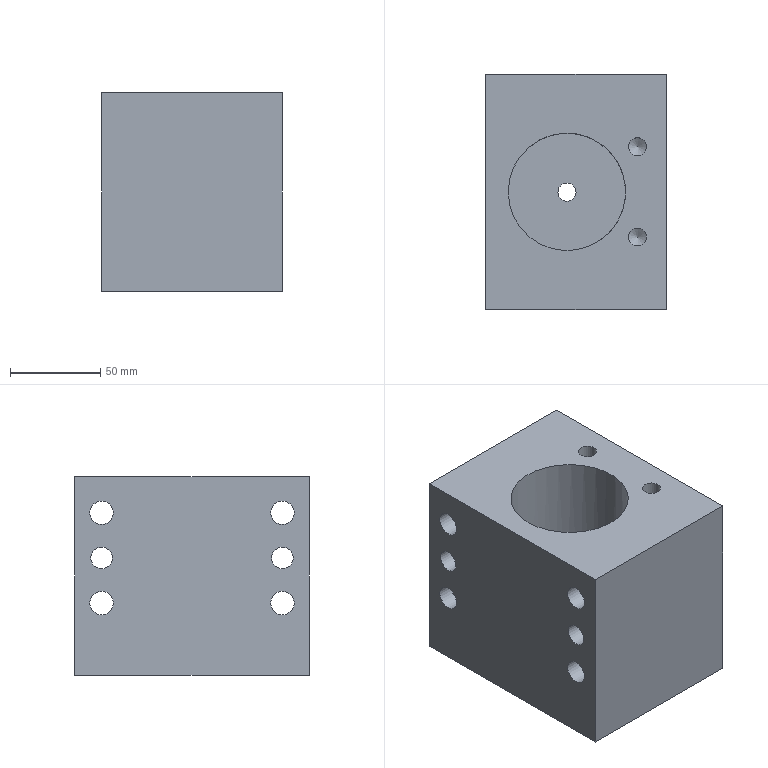Part | NX | features solid 2 | 1 solid | 31 faces | box 100 x 130 x 110 mm | volume 972878 mm3 | cylinder 16 | plane 13 | cone 2 | commonest cylinder face diameters 13 x4 20 x4 10 x3 12 x2 14 x2 65 x1
STEP:
#1=CARTESIAN_POINT('',(670.,65.,-145.));
#2=VERTEX_POINT('',#1);
#3=CARTESIAN_POINT('',(670.,65.,-152.));
#4=DIRECTION('',(-1.,0.,0.));
#5=DIRECTION('',(0.,0.,1.));
#6=AXIS2_PLACEMENT_3D('',#3,#4,#5);
#7=CIRCLE('',#6,7.);
#8=EDGE_CURVE('',#2,#2,#7,.F.);
#9=ORIENTED_EDGE('',*,*,#8,.F.);
#10=EDGE_LOOP('',(#9));
#11=FACE_BOUND('',#10,.T.);
#12=CARTESIAN_POINT('',(670.,165.,-117.));
#13=VERTEX_POINT('',#12);
#14=CARTESIAN_POINT('',(670.,165.,-127.));
#15=DIRECTION('',(-1.,0.,0.));
#16=DIRECTION('',(0.,0.,1.));
#17=AXIS2_PLACEMENT_3D('',#14,#15,#16);
#18=CIRCLE('',#17,10.);
#19=EDGE_CURVE('',#13,#13,#18,.T.);
#20=ORIENTED_EDGE('',*,*,#19,.T.);
#21=EDGE_LOOP('',(#20));
#22=FACE_BOUND('',#21,.T.);
#23=CARTESIAN_POINT('',(670.,165.,-167.));
#24=VERTEX_POINT('',#23);
#25=CARTESIAN_POINT('',(670.,165.,-177.));
#26=DIRECTION('',(-1.,0.,0.));
#27=DIRECTION('',(0.,0.,1.));
#28=AXIS2_PLACEMENT_3D('',#25,#26,#27);
#29=CIRCLE('',#28,10.);
#30=EDGE_CURVE('',#24,#24,#29,.T.);
#31=ORIENTED_EDGE('',*,*,#30,.T.);
#32=EDGE_LOOP('',(#31));
#33=FACE_BOUND('',#32,.T.);
#34=CARTESIAN_POINT('',(670.,65.,-167.));
#35=VERTEX_POINT('',#34);
#36=CARTESIAN_POINT('',(670.,65.,-177.));
#37=DIRECTION('',(-1.,0.,0.));
#38=DIRECTION('',(0.,0.,1.));
#39=AXIS2_PLACEMENT_3D('',#36,#37,#38);
#40=CIRCLE('',#39,10.);
#41=EDGE_CURVE('',#35,#35,#40,.T.);
#42=ORIENTED_EDGE('',*,*,#41,.T.);
#43=EDGE_LOOP('',(#42));
#44=FACE_BOUND('',#43,.T.);
#45=CARTESIAN_POINT('',(670.,65.,-117.));
#46=VERTEX_POINT('',#45);
#47=CARTESIAN_POINT('',(670.,65.,-127.));
#48=DIRECTION('',(-1.,0.,0.));
#49=DIRECTION('',(0.,0.,1.));
#50=AXIS2_PLACEMENT_3D('',#47,#48,#49);
#51=CIRCLE('',#50,10.);
#52=EDGE_CURVE('',#46,#46,#51,.T.);
#53=ORIENTED_EDGE('',*,*,#52,.T.);
#54=EDGE_LOOP('',(#53));
#55=FACE_BOUND('',#54,.T.);
#56=CARTESIAN_POINT('',(670.,180.,-107.));
#57=VERTEX_POINT('',#56);
#58=CARTESIAN_POINT('',(670.,50.,-107.));
#59=VERTEX_POINT('',#58);
#60=CARTESIAN_POINT('',(670.,180.,-107.));
#61=DIRECTION('',(0.,-1.,0.));
#62=VECTOR('',#61,1000.);
#63=LINE('',#60,#62);
#64=EDGE_CURVE('',#57,#59,#63,.T.);
#65=ORIENTED_EDGE('',*,*,#64,.T.);
#66=CARTESIAN_POINT('',(670.,50.,-217.));
#67=VERTEX_POINT('',#66);
#68=CARTESIAN_POINT('',(670.,50.,-210.));
#69=DIRECTION('',(0.,0.,1.));
#70=VECTOR('',#69,1000.);
#71=LINE('',#68,#70);
#72=EDGE_CURVE('',#67,#59,#71,.T.);
#73=ORIENTED_EDGE('',*,*,#72,.F.);
#74=CARTESIAN_POINT('',(670.,180.,-217.));
#75=VERTEX_POINT('',#74);
#76=CARTESIAN_POINT('',(670.,180.,-217.));
#77=DIRECTION('',(0.,1.,0.));
#78=VECTOR('',#77,1000.);
#79=LINE('',#76,#78);
#80=EDGE_CURVE('',#75,#67,#79,.F.);
#81=ORIENTED_EDGE('',*,*,#80,.F.);
#82=CARTESIAN_POINT('',(670.,180.,-210.));
#83=DIRECTION('',(0.,0.,1.));
#84=VECTOR('',#83,1000.);
#85=LINE('',#82,#84);
#86=EDGE_CURVE('',#75,#57,#85,.T.);
#87=ORIENTED_EDGE('',*,*,#86,.T.);
#88=EDGE_LOOP('',(#65,#73,#81,#87));
#89=FACE_BOUND('',#88,.T.);
#90=CARTESIAN_POINT('',(670.,165.,-145.));
#91=VERTEX_POINT('',#90);
#92=CARTESIAN_POINT('',(670.,165.,-152.));
#93=DIRECTION('',(-1.,0.,0.));
#94=DIRECTION('',(0.,0.,1.));
#95=AXIS2_PLACEMENT_3D('',#92,#93,#94);
#96=CIRCLE('',#95,7.);
#97=EDGE_CURVE('',#91,#91,#96,.F.);
#98=ORIENTED_EDGE('',*,*,#97,.F.);
#99=EDGE_LOOP('',(#98));
#100=FACE_BOUND('',#99,.T.);
#101=CARTESIAN_POINT('',(670.,180.,-210.));
#102=DIRECTION('',(-1.,0.,0.));
#103=DIRECTION('',(0.,0.,1.));
#104=AXIS2_PLACEMENT_3D('',#101,#102,#103);
#105=PLANE('',#104);
#106=ADVANCED_FACE('',(#11,#22,#33,#44,#55,#89,#100),#105,.F.);
#107=CARTESIAN_POINT('',(570.,165.,-146.));
#108=VERTEX_POINT('',#107);
#109=CARTESIAN_POINT('',(570.,165.,-152.));
#110=DIRECTION('',(-1.,0.,0.));
#111=DIRECTION('',(0.,0.,1.));
#112=AXIS2_PLACEMENT_3D('',#109,#110,#111);
#113=CIRCLE('',#112,6.);
#114=EDGE_CURVE('',#108,#108,#113,.F.);
#115=ORIENTED_EDGE('',*,*,#114,.F.);
#116=EDGE_LOOP('',(#115));
#117=FACE_BOUND('',#116,.T.);
#118=CARTESIAN_POINT('',(610.,165.,-158.));
#119=VERTEX_POINT('',#118);
#120=CARTESIAN_POINT('',(610.,165.,-152.));
#121=DIRECTION('',(1.,0.,0.));
#122=DIRECTION('',(0.,0.,-1.));
#123=AXIS2_PLACEMENT_3D('',#120,#121,#122);
#124=CIRCLE('',#123,6.);
#125=EDGE_CURVE('',#119,#119,#124,.T.);
#126=ORIENTED_EDGE('',*,*,#125,.T.);
#127=EDGE_LOOP('',(#126));
#128=FACE_BOUND('',#127,.T.);
#129=CARTESIAN_POINT('',(505.,165.,-152.));
#130=DIRECTION('',(1.,0.,0.));
#131=DIRECTION('',(0.,0.,-1.));
#132=AXIS2_PLACEMENT_3D('',#129,#130,#131);
#133=CYLINDRICAL_SURFACE('',#132,6.);
#134=ADVANCED_FACE('',(#117,#128),#133,.F.);
#135=CARTESIAN_POINT('',(570.,65.,-146.));
#136=VERTEX_POINT('',#135);
#137=CARTESIAN_POINT('',(570.,65.,-152.));
#138=DIRECTION('',(-1.,0.,0.));
#139=DIRECTION('',(0.,0.,1.));
#140=AXIS2_PLACEMENT_3D('',#137,#138,#139);
#141=CIRCLE('',#140,6.);
#142=EDGE_CURVE('',#136,#136,#141,.F.);
#143=ORIENTED_EDGE('',*,*,#142,.F.);
#144=EDGE_LOOP('',(#143));
#145=FACE_BOUND('',#144,.T.);
#146=CARTESIAN_POINT('',(610.,65.,-158.));
#147=VERTEX_POINT('',#146);
#148=CARTESIAN_POINT('',(610.,65.,-152.));
#149=DIRECTION('',(1.,0.,0.));
#150=DIRECTION('',(0.,0.,-1.));
#151=AXIS2_PLACEMENT_3D('',#148,#149,#150);
#152=CIRCLE('',#151,6.);
#153=EDGE_CURVE('',#147,#147,#152,.T.);
#154=ORIENTED_EDGE('',*,*,#153,.T.);
#155=EDGE_LOOP('',(#154));
#156=FACE_BOUND('',#155,.T.);
#157=CARTESIAN_POINT('',(505.,65.,-152.));
#158=DIRECTION('',(1.,0.,0.));
#159=DIRECTION('',(0.,0.,-1.));
#160=AXIS2_PLACEMENT_3D('',#157,#158,#159);
#161=CYLINDRICAL_SURFACE('',#160,6.);
#162=ADVANCED_FACE('',(#145,#156),#161,.F.);
#163=ORIENTED_EDGE('',*,*,#142,.T.);
#164=EDGE_LOOP('',(#163));
#165=FACE_BOUND('',#164,.T.);
#166=CARTESIAN_POINT('',(570.,165.,-120.5));
#167=VERTEX_POINT('',#166);
#168=CARTESIAN_POINT('',(570.,165.,-127.));
#169=DIRECTION('',(-1.,0.,0.));
#170=DIRECTION('',(0.,0.,1.));
#171=AXIS2_PLACEMENT_3D('',#168,#169,#170);
#172=CIRCLE('',#171,6.5);
#173=EDGE_CURVE('',#167,#167,#172,.T.);
#174=ORIENTED_EDGE('',*,*,#173,.F.);
#175=EDGE_LOOP('',(#174));
#176=FACE_BOUND('',#175,.T.);
#177=CARTESIAN_POINT('',(570.,165.,-170.5));
#178=VERTEX_POINT('',#177);
#179=CARTESIAN_POINT('',(570.,165.,-177.));
#180=DIRECTION('',(-1.,0.,0.));
#181=DIRECTION('',(0.,0.,1.));
#182=AXIS2_PLACEMENT_3D('',#179,#180,#181);
#183=CIRCLE('',#182,6.5);
#184=EDGE_CURVE('',#178,#178,#183,.T.);
#185=ORIENTED_EDGE('',*,*,#184,.F.);
#186=EDGE_LOOP('',(#185));
#187=FACE_BOUND('',#186,.T.);
#188=CARTESIAN_POINT('',(570.,65.,-170.5));
#189=VERTEX_POINT('',#188);
#190=CARTESIAN_POINT('',(570.,65.,-177.));
#191=DIRECTION('',(-1.,0.,0.));
#192=DIRECTION('',(0.,0.,1.));
#193=AXIS2_PLACEMENT_3D('',#190,#191,#192);
#194=CIRCLE('',#193,6.5);
#195=EDGE_CURVE('',#189,#189,#194,.T.);
#196=ORIENTED_EDGE('',*,*,#195,.F.);
#197=EDGE_LOOP('',(#196));
#198=FACE_BOUND('',#197,.T.);
#199=CARTESIAN_POINT('',(570.,65.,-120.5));
#200=VERTEX_POINT('',#199);
#201=CARTESIAN_POINT('',(570.,65.,-127.));
#202=DIRECTION('',(-1.,0.,0.));
#203=DIRECTION('',(0.,0.,1.));
#204=AXIS2_PLACEMENT_3D('',#201,#202,#203);
#205=CIRCLE('',#204,6.5);
#206=EDGE_CURVE('',#200,#200,#205,.T.);
#207=ORIENTED_EDGE('',*,*,#206,.F.);
#208=EDGE_LOOP('',(#207));
#209=FACE_BOUND('',#208,.T.);
#210=CARTESIAN_POINT('',(570.,180.,-107.));
#211=VERTEX_POINT('',#210);
#212=CARTESIAN_POINT('',(570.,50.,-107.));
#213=VERTEX_POINT('',#212);
#214=CARTESIAN_POINT('',(570.,180.,-107.));
#215=DIRECTION('',(0.,-1.,0.));
#216=VECTOR('',#215,1000.);
#217=LINE('',#214,#216);
#218=EDGE_CURVE('',#211,#213,#217,.T.);
#219=ORIENTED_EDGE('',*,*,#218,.F.);
#220=CARTESIAN_POINT('',(570.,180.,-217.));
#221=VERTEX_POINT('',#220);
#222=CARTESIAN_POINT('',(570.,180.,-210.));
#223=DIRECTION('',(0.,0.,1.));
#224=VECTOR('',#223,1000.);
#225=LINE('',#222,#224);
#226=EDGE_CURVE('',#221,#211,#225,.T.);
#227=ORIENTED_EDGE('',*,*,#226,.F.);
#228=CARTESIAN_POINT('',(570.,50.,-217.));
#229=VERTEX_POINT('',#228);
#230=CARTESIAN_POINT('',(570.,180.,-217.));
#231=DIRECTION('',(0.,1.,0.));
#232=VECTOR('',#231,1000.);
#233=LINE('',#230,#232);
#234=EDGE_CURVE('',#221,#229,#233,.F.);
#235=ORIENTED_EDGE('',*,*,#234,.T.);
#236=CARTESIAN_POINT('',(570.,50.,-210.));
#237=DIRECTION('',(0.,0.,1.));
#238=VECTOR('',#237,1000.);
#239=LINE('',#236,#238);
#240=EDGE_CURVE('',#229,#213,#239,.T.);
#241=ORIENTED_EDGE('',*,*,#240,.T.);
#242=EDGE_LOOP('',(#219,#227,#235,#241));
#243=FACE_BOUND('',#242,.T.);
#244=ORIENTED_EDGE('',*,*,#114,.T.);
#245=EDGE_LOOP('',(#244));
#246=FACE_BOUND('',#245,.T.);
#247=CARTESIAN_POINT('',(570.,180.,-210.));
#248=DIRECTION('',(-1.,0.,0.));
#249=DIRECTION('',(0.,0.,1.));
#250=AXIS2_PLACEMENT_3D('',#247,#248,#249);
#251=PLANE('',#250);
#252=ADVANCED_FACE('',(#165,#176,#187,#198,#209,#243,#246),#251,.T.);
#253=CARTESIAN_POINT('',(610.,115.,-217.));
#254=VERTEX_POINT('',#253);
#255=CARTESIAN_POINT('',(615.,115.,-217.));
#256=DIRECTION('',(0.,0.,-1.));
#257=DIRECTION('',(-1.,0.,0.));
#258=AXIS2_PLACEMENT_3D('',#255,#256,#257);
#259=CIRCLE('',#258,5.);
#260=EDGE_CURVE('',#254,#254,#259,.F.);
#261=ORIENTED_EDGE('',*,*,#260,.T.);
#262=EDGE_LOOP('',(#261));
#263=FACE_BOUND('',#262,.T.);
#264=CARTESIAN_POINT('',(570.,180.,-217.));
#265=DIRECTION('',(-1.,0.,0.));
#266=VECTOR('',#265,1000.);
#267=LINE('',#264,#266);
#268=EDGE_CURVE('',#221,#75,#267,.F.);
#269=ORIENTED_EDGE('',*,*,#268,.T.);
#270=ORIENTED_EDGE('',*,*,#80,.T.);
#271=CARTESIAN_POINT('',(570.,50.,-217.));
#272=DIRECTION('',(1.,0.,0.));
#273=VECTOR('',#272,1000.);
#274=LINE('',#271,#273);
#275=EDGE_CURVE('',#229,#67,#274,.T.);
#276=ORIENTED_EDGE('',*,*,#275,.F.);
#277=ORIENTED_EDGE('',*,*,#234,.F.);
#278=EDGE_LOOP('',(#269,#270,#276,#277));
#279=FACE_BOUND('',#278,.T.);
#280=CARTESIAN_POINT('',(570.,180.,-217.));
#281=DIRECTION('',(0.,0.,-1.));
#282=DIRECTION('',(0.,-1.,0.));
#283=AXIS2_PLACEMENT_3D('',#280,#281,#282);
#284=PLANE('',#283);
#285=ADVANCED_FACE('',(#263,#279),#284,.T.);
#286=ORIENTED_EDGE('',*,*,#275,.T.);
#287=ORIENTED_EDGE('',*,*,#72,.T.);
#288=CARTESIAN_POINT('',(640.,50.,-107.));
#289=DIRECTION('',(-1.,0.,0.));
#290=VECTOR('',#289,1000.);
#291=LINE('',#288,#290);
#292=EDGE_CURVE('',#213,#59,#291,.F.);
#293=ORIENTED_EDGE('',*,*,#292,.F.);
#294=ORIENTED_EDGE('',*,*,#240,.F.);
#295=EDGE_LOOP('',(#286,#287,#293,#294));
#296=FACE_BOUND('',#295,.T.);
#297=CARTESIAN_POINT('',(570.,50.,-210.));
#298=DIRECTION('',(0.,-1.,0.));
#299=DIRECTION('',(0.,0.,1.));
#300=AXIS2_PLACEMENT_3D('',#297,#298,#299);
#301=PLANE('',#300);
#302=ADVANCED_FACE('',(#296),#301,.T.);
#303=CARTESIAN_POINT('',(649.,140.,-107.));
#304=VERTEX_POINT('',#303);
#305=CARTESIAN_POINT('',(654.,140.,-107.));
#306=DIRECTION('',(0.,0.,-1.));
#307=DIRECTION('',(-1.,0.,0.));
#308=AXIS2_PLACEMENT_3D('',#305,#306,#307);
#309=CIRCLE('',#308,5.);
#310=EDGE_CURVE('',#304,#304,#309,.T.);
#311=ORIENTED_EDGE('',*,*,#310,.T.);
#312=EDGE_LOOP('',(#311));
#313=FACE_BOUND('',#312,.T.);
#314=CARTESIAN_POINT('',(649.,90.,-107.));
#315=VERTEX_POINT('',#314);
#316=CARTESIAN_POINT('',(654.,90.,-107.));
#317=DIRECTION('',(0.,0.,-1.));
#318=DIRECTION('',(-1.,0.,0.));
#319=AXIS2_PLACEMENT_3D('',#316,#317,#318);
#320=CIRCLE('',#319,5.);
#321=EDGE_CURVE('',#315,#315,#320,.T.);
#322=ORIENTED_EDGE('',*,*,#321,.T.);
#323=EDGE_LOOP('',(#322));
#324=FACE_BOUND('',#323,.T.);
#325=CARTESIAN_POINT('',(582.5,115.,-107.));
#326=VERTEX_POINT('',#325);
#327=CARTESIAN_POINT('',(615.,115.,-107.));
#328=DIRECTION('',(0.,0.,-1.));
#329=DIRECTION('',(-1.,0.,0.));
#330=AXIS2_PLACEMENT_3D('',#327,#328,#329);
#331=CIRCLE('',#330,32.5);
#332=EDGE_CURVE('',#326,#326,#331,.T.);
#333=ORIENTED_EDGE('',*,*,#332,.T.);
#334=EDGE_LOOP('',(#333));
#335=FACE_BOUND('',#334,.T.);
#336=ORIENTED_EDGE('',*,*,#292,.T.);
#337=ORIENTED_EDGE('',*,*,#64,.F.);
#338=CARTESIAN_POINT('',(570.,180.,-107.));
#339=DIRECTION('',(1.,0.,0.));
#340=VECTOR('',#339,1000.);
#341=LINE('',#338,#340);
#342=EDGE_CURVE('',#211,#57,#341,.T.);
#343=ORIENTED_EDGE('',*,*,#342,.F.);
#344=ORIENTED_EDGE('',*,*,#218,.T.);
#345=EDGE_LOOP('',(#336,#337,#343,#344));
#346=FACE_BOUND('',#345,.T.);
#347=CARTESIAN_POINT('',(640.,75.,-107.));
#348=DIRECTION('',(0.,0.,-1.));
#349=DIRECTION('',(0.,1.,0.));
#350=AXIS2_PLACEMENT_3D('',#347,#348,#349);
#351=PLANE('',#350);
#352=ADVANCED_FACE('',(#313,#324,#335,#346),#351,.F.);
#353=ORIENTED_EDGE('',*,*,#226,.T.);
#354=ORIENTED_EDGE('',*,*,#342,.T.);
#355=ORIENTED_EDGE('',*,*,#86,.F.);
#356=ORIENTED_EDGE('',*,*,#268,.F.);
#357=EDGE_LOOP('',(#353,#354,#355,#356));
#358=FACE_BOUND('',#357,.T.);
#359=CARTESIAN_POINT('',(570.,180.,-210.));
#360=DIRECTION('',(0.,-1.,0.));
#361=DIRECTION('',(0.,0.,1.));
#362=AXIS2_PLACEMENT_3D('',#359,#360,#361);
#363=PLANE('',#362);
#364=ADVANCED_FACE('',(#358),#363,.F.);
#365=CARTESIAN_POINT('',(647.5,115.,-204.));
#366=VERTEX_POINT('',#365);
#367=CARTESIAN_POINT('',(615.,115.,-204.));
#368=DIRECTION('',(0.,0.,-1.));
#369=DIRECTION('',(1.,0.,0.));
#370=AXIS2_PLACEMENT_3D('',#367,#368,#369);
#371=CIRCLE('',#370,32.5);
#372=EDGE_CURVE('',#366,#366,#371,.T.);
#373=ORIENTED_EDGE('',*,*,#372,.T.);
#374=EDGE_LOOP('',(#373));
#375=FACE_BOUND('',#374,.T.);
#376=ORIENTED_EDGE('',*,*,#332,.F.);
#377=EDGE_LOOP('',(#376));
#378=FACE_BOUND('',#377,.T.);
#379=CARTESIAN_POINT('',(615.,115.,-99.));
#380=DIRECTION('',(0.,0.,-1.));
#381=DIRECTION('',(-1.,0.,0.));
#382=AXIS2_PLACEMENT_3D('',#379,#380,#381);
#383=CYLINDRICAL_SURFACE('',#382,32.5);
#384=ADVANCED_FACE('',(#375,#378),#383,.F.);
#385=CARTESIAN_POINT('',(610.,115.,-204.));
#386=VERTEX_POINT('',#385);
#387=CARTESIAN_POINT('',(615.,115.,-204.));
#388=DIRECTION('',(0.,0.,-1.));
#389=DIRECTION('',(-1.,0.,0.));
#390=AXIS2_PLACEMENT_3D('',#387,#388,#389);
#391=CIRCLE('',#390,5.);
#392=EDGE_CURVE('',#386,#386,#391,.T.);
#393=ORIENTED_EDGE('',*,*,#392,.T.);
#394=EDGE_LOOP('',(#393));
#395=FACE_BOUND('',#394,.T.);
#396=ORIENTED_EDGE('',*,*,#372,.F.);
#397=EDGE_LOOP('',(#396));
#398=FACE_BOUND('',#397,.T.);
#399=CARTESIAN_POINT('',(615.,115.,-204.));
#400=DIRECTION('',(0.,0.,-1.));
#401=DIRECTION('',(-1.,0.,0.));
#402=AXIS2_PLACEMENT_3D('',#399,#400,#401);
#403=PLANE('',#402);
#404=ADVANCED_FACE('',(#395,#398),#403,.F.);
#405=CARTESIAN_POINT('',(605.,65.,-137.));
#406=VERTEX_POINT('',#405);
#407=CARTESIAN_POINT('',(605.,65.,-127.));
#408=DIRECTION('',(1.,0.,0.));
#409=DIRECTION('',(0.,0.,-1.));
#410=AXIS2_PLACEMENT_3D('',#407,#408,#409);
#411=CIRCLE('',#410,10.);
#412=EDGE_CURVE('',#406,#406,#411,.T.);
#413=ORIENTED_EDGE('',*,*,#412,.F.);
#414=EDGE_LOOP('',(#413));
#415=FACE_BOUND('',#414,.T.);
#416=ORIENTED_EDGE('',*,*,#52,.F.);
#417=EDGE_LOOP('',(#416));
#418=FACE_BOUND('',#417,.T.);
#419=CARTESIAN_POINT('',(605.,65.,-127.));
#420=DIRECTION('',(1.,0.,0.));
#421=DIRECTION('',(0.,0.,-1.));
#422=AXIS2_PLACEMENT_3D('',#419,#420,#421);
#423=CYLINDRICAL_SURFACE('',#422,10.);
#424=ADVANCED_FACE('',(#415,#418),#423,.F.);
#425=ORIENTED_EDGE('',*,*,#206,.T.);
#426=EDGE_LOOP('',(#425));
#427=FACE_BOUND('',#426,.T.);
#428=CARTESIAN_POINT('',(605.,65.,-120.5));
#429=VERTEX_POINT('',#428);
#430=CARTESIAN_POINT('',(605.,65.,-127.));
#431=DIRECTION('',(-1.,0.,0.));
#432=DIRECTION('',(0.,0.,1.));
#433=AXIS2_PLACEMENT_3D('',#430,#431,#432);
#434=CIRCLE('',#433,6.5);
#435=EDGE_CURVE('',#429,#429,#434,.F.);
#436=ORIENTED_EDGE('',*,*,#435,.T.);
#437=EDGE_LOOP('',(#436));
#438=FACE_BOUND('',#437,.T.);
#439=CARTESIAN_POINT('',(535.,65.,-127.));
#440=DIRECTION('',(1.,0.,0.));
#441=DIRECTION('',(0.,0.,-1.));
#442=AXIS2_PLACEMENT_3D('',#439,#440,#441);
#443=CYLINDRICAL_SURFACE('',#442,6.5);
#444=ADVANCED_FACE('',(#427,#438),#443,.F.);
#445=ORIENTED_EDGE('',*,*,#435,.F.);
#446=EDGE_LOOP('',(#445));
#447=FACE_BOUND('',#446,.T.);
#448=ORIENTED_EDGE('',*,*,#412,.T.);
#449=EDGE_LOOP('',(#448));
#450=FACE_BOUND('',#449,.T.);
#451=CARTESIAN_POINT('',(605.,65.,-127.));
#452=DIRECTION('',(-1.,0.,0.));
#453=DIRECTION('',(0.,0.,1.));
#454=AXIS2_PLACEMENT_3D('',#451,#452,#453);
#455=PLANE('',#454);
#456=ADVANCED_FACE('',(#447,#450),#455,.F.);
#457=CARTESIAN_POINT('',(605.,65.,-187.));
#458=VERTEX_POINT('',#457);
#459=CARTESIAN_POINT('',(605.,65.,-177.));
#460=DIRECTION('',(1.,0.,0.));
#461=DIRECTION('',(0.,0.,-1.));
#462=AXIS2_PLACEMENT_3D('',#459,#460,#461);
#463=CIRCLE('',#462,10.);
#464=EDGE_CURVE('',#458,#458,#463,.T.);
#465=ORIENTED_EDGE('',*,*,#464,.F.);
#466=EDGE_LOOP('',(#465));
#467=FACE_BOUND('',#466,.T.);
#468=ORIENTED_EDGE('',*,*,#41,.F.);
#469=EDGE_LOOP('',(#468));
#470=FACE_BOUND('',#469,.T.);
#471=CARTESIAN_POINT('',(605.,65.,-177.));
#472=DIRECTION('',(1.,0.,0.));
#473=DIRECTION('',(0.,0.,-1.));
#474=AXIS2_PLACEMENT_3D('',#471,#472,#473);
#475=CYLINDRICAL_SURFACE('',#474,10.);
#476=ADVANCED_FACE('',(#467,#470),#475,.F.);
#477=ORIENTED_EDGE('',*,*,#195,.T.);
#478=EDGE_LOOP('',(#477));
#479=FACE_BOUND('',#478,.T.);
#480=CARTESIAN_POINT('',(605.,65.,-170.5));
#481=VERTEX_POINT('',#480);
#482=CARTESIAN_POINT('',(605.,65.,-177.));
#483=DIRECTION('',(-1.,0.,0.));
#484=DIRECTION('',(0.,0.,1.));
#485=AXIS2_PLACEMENT_3D('',#482,#483,#484);
#486=CIRCLE('',#485,6.5);
#487=EDGE_CURVE('',#481,#481,#486,.F.);
#488=ORIENTED_EDGE('',*,*,#487,.T.);
#489=EDGE_LOOP('',(#488));
#490=FACE_BOUND('',#489,.T.);
#491=CARTESIAN_POINT('',(535.,65.,-177.));
#492=DIRECTION('',(1.,0.,0.));
#493=DIRECTION('',(0.,0.,-1.));
#494=AXIS2_PLACEMENT_3D('',#491,#492,#493);
#495=CYLINDRICAL_SURFACE('',#494,6.5);
#496=ADVANCED_FACE('',(#479,#490),#495,.F.);
#497=ORIENTED_EDGE('',*,*,#487,.F.);
#498=EDGE_LOOP('',(#497));
#499=FACE_BOUND('',#498,.T.);
#500=ORIENTED_EDGE('',*,*,#464,.T.);
#501=EDGE_LOOP('',(#500));
#502=FACE_BOUND('',#501,.T.);
#503=CARTESIAN_POINT('',(605.,65.,-177.));
#504=DIRECTION('',(-1.,0.,0.));
#505=DIRECTION('',(0.,0.,1.));
#506=AXIS2_PLACEMENT_3D('',#503,#504,#505);
#507=PLANE('',#506);
#508=ADVANCED_FACE('',(#499,#502),#507,.F.);
#509=CARTESIAN_POINT('',(605.,165.,-187.));
#510=VERTEX_POINT('',#509);
#511=CARTESIAN_POINT('',(605.,165.,-177.));
#512=DIRECTION('',(1.,0.,0.));
#513=DIRECTION('',(0.,0.,-1.));
#514=AXIS2_PLACEMENT_3D('',#511,#512,#513);
#515=CIRCLE('',#514,10.);
#516=EDGE_CURVE('',#510,#510,#515,.T.);
#517=ORIENTED_EDGE('',*,*,#516,.F.);
#518=EDGE_LOOP('',(#517));
#519=FACE_BOUND('',#518,.T.);
#520=ORIENTED_EDGE('',*,*,#30,.F.);
#521=EDGE_LOOP('',(#520));
#522=FACE_BOUND('',#521,.T.);
#523=CARTESIAN_POINT('',(605.,165.,-177.));
#524=DIRECTION('',(1.,0.,0.));
#525=DIRECTION('',(0.,0.,-1.));
#526=AXIS2_PLACEMENT_3D('',#523,#524,#525);
#527=CYLINDRICAL_SURFACE('',#526,10.);
#528=ADVANCED_FACE('',(#519,#522),#527,.F.);
#529=ORIENTED_EDGE('',*,*,#184,.T.);
#530=EDGE_LOOP('',(#529));
#531=FACE_BOUND('',#530,.T.);
#532=CARTESIAN_POINT('',(605.,165.,-170.5));
#533=VERTEX_POINT('',#532);
#534=CARTESIAN_POINT('',(605.,165.,-177.));
#535=DIRECTION('',(-1.,0.,0.));
#536=DIRECTION('',(0.,0.,1.));
#537=AXIS2_PLACEMENT_3D('',#534,#535,#536);
#538=CIRCLE('',#537,6.5);
#539=EDGE_CURVE('',#533,#533,#538,.F.);
#540=ORIENTED_EDGE('',*,*,#539,.T.);
#541=EDGE_LOOP('',(#540));
#542=FACE_BOUND('',#541,.T.);
#543=CARTESIAN_POINT('',(535.,165.,-177.));
#544=DIRECTION('',(1.,0.,0.));
#545=DIRECTION('',(0.,0.,-1.));
#546=AXIS2_PLACEMENT_3D('',#543,#544,#545);
#547=CYLINDRICAL_SURFACE('',#546,6.5);
#548=ADVANCED_FACE('',(#531,#542),#547,.F.);
#549=ORIENTED_EDGE('',*,*,#539,.F.);
#550=EDGE_LOOP('',(#549));
#551=FACE_BOUND('',#550,.T.);
#552=ORIENTED_EDGE('',*,*,#516,.T.);
#553=EDGE_LOOP('',(#552));
#554=FACE_BOUND('',#553,.T.);
#555=CARTESIAN_POINT('',(605.,165.,-177.));
#556=DIRECTION('',(-1.,0.,0.));
#557=DIRECTION('',(0.,0.,1.));
#558=AXIS2_PLACEMENT_3D('',#555,#556,#557);
#559=PLANE('',#558);
#560=ADVANCED_FACE('',(#551,#554),#559,.F.);
#561=CARTESIAN_POINT('',(605.,165.,-137.));
#562=VERTEX_POINT('',#561);
#563=CARTESIAN_POINT('',(605.,165.,-127.));
#564=DIRECTION('',(1.,0.,0.));
#565=DIRECTION('',(0.,0.,-1.));
#566=AXIS2_PLACEMENT_3D('',#563,#564,#565);
#567=CIRCLE('',#566,10.);
#568=EDGE_CURVE('',#562,#562,#567,.T.);
#569=ORIENTED_EDGE('',*,*,#568,.F.);
#570=EDGE_LOOP('',(#569));
#571=FACE_BOUND('',#570,.T.);
#572=ORIENTED_EDGE('',*,*,#19,.F.);
#573=EDGE_LOOP('',(#572));
#574=FACE_BOUND('',#573,.T.);
#575=CARTESIAN_POINT('',(605.,165.,-127.));
#576=DIRECTION('',(1.,0.,0.));
#577=DIRECTION('',(0.,0.,-1.));
#578=AXIS2_PLACEMENT_3D('',#575,#576,#577);
#579=CYLINDRICAL_SURFACE('',#578,10.);
#580=ADVANCED_FACE('',(#571,#574),#579,.F.);
#581=ORIENTED_EDGE('',*,*,#173,.T.);
#582=EDGE_LOOP('',(#581));
#583=FACE_BOUND('',#582,.T.);
#584=CARTESIAN_POINT('',(605.,165.,-120.5));
#585=VERTEX_POINT('',#584);
#586=CARTESIAN_POINT('',(605.,165.,-127.));
#587=DIRECTION('',(-1.,0.,0.));
#588=DIRECTION('',(0.,0.,1.));
#589=AXIS2_PLACEMENT_3D('',#586,#587,#588);
#590=CIRCLE('',#589,6.5);
#591=EDGE_CURVE('',#585,#585,#590,.F.);
#592=ORIENTED_EDGE('',*,*,#591,.T.);
#593=EDGE_LOOP('',(#592));
#594=FACE_BOUND('',#593,.T.);
#595=CARTESIAN_POINT('',(535.,165.,-127.));
#596=DIRECTION('',(1.,0.,0.));
#597=DIRECTION('',(0.,0.,-1.));
#598=AXIS2_PLACEMENT_3D('',#595,#596,#597);
#599=CYLINDRICAL_SURFACE('',#598,6.5);
#600=ADVANCED_FACE('',(#583,#594),#599,.F.);
#601=ORIENTED_EDGE('',*,*,#591,.F.);
#602=EDGE_LOOP('',(#601));
#603=FACE_BOUND('',#602,.T.);
#604=ORIENTED_EDGE('',*,*,#568,.T.);
#605=EDGE_LOOP('',(#604));
#606=FACE_BOUND('',#605,.T.);
#607=CARTESIAN_POINT('',(605.,165.,-127.));
#608=DIRECTION('',(-1.,0.,0.));
#609=DIRECTION('',(0.,0.,1.));
#610=AXIS2_PLACEMENT_3D('',#607,#608,#609);
#611=PLANE('',#610);
#612=ADVANCED_FACE('',(#603,#606),#611,.F.);
#613=CARTESIAN_POINT('',(610.,65.,-159.));
#614=VERTEX_POINT('',#613);
#615=CARTESIAN_POINT('',(610.,65.,-152.));
#616=DIRECTION('',(1.,0.,0.));
#617=DIRECTION('',(0.,0.,-1.));
#618=AXIS2_PLACEMENT_3D('',#615,#616,#617);
#619=CIRCLE('',#618,7.);
#620=EDGE_CURVE('',#614,#614,#619,.T.);
#621=ORIENTED_EDGE('',*,*,#620,.F.);
#622=EDGE_LOOP('',(#621));
#623=FACE_BOUND('',#622,.T.);
#624=ORIENTED_EDGE('',*,*,#8,.T.);
#625=EDGE_LOOP('',(#624));
#626=FACE_BOUND('',#625,.T.);
#627=CARTESIAN_POINT('',(770.,65.,-152.));
#628=DIRECTION('',(-1.,0.,0.));
#629=DIRECTION('',(0.,0.,1.));
#630=AXIS2_PLACEMENT_3D('',#627,#628,#629);
#631=CYLINDRICAL_SURFACE('',#630,7.);
#632=ADVANCED_FACE('',(#623,#626),#631,.F.);
#633=ORIENTED_EDGE('',*,*,#153,.F.);
#634=EDGE_LOOP('',(#633));
#635=FACE_BOUND('',#634,.T.);
#636=ORIENTED_EDGE('',*,*,#620,.T.);
#637=EDGE_LOOP('',(#636));
#638=FACE_BOUND('',#637,.T.);
#639=CARTESIAN_POINT('',(610.,65.,-152.));
#640=DIRECTION('',(1.,0.,0.));
#641=DIRECTION('',(0.,0.,-1.));
#642=AXIS2_PLACEMENT_3D('',#639,#640,#641);
#643=PLANE('',#642);
#644=ADVANCED_FACE('',(#635,#638),#643,.T.);
#645=CARTESIAN_POINT('',(610.,165.,-159.));
#646=VERTEX_POINT('',#645);
#647=CARTESIAN_POINT('',(610.,165.,-152.));
#648=DIRECTION('',(1.,0.,0.));
#649=DIRECTION('',(0.,0.,-1.));
#650=AXIS2_PLACEMENT_3D('',#647,#648,#649);
#651=CIRCLE('',#650,7.);
#652=EDGE_CURVE('',#646,#646,#651,.T.);
#653=ORIENTED_EDGE('',*,*,#652,.F.);
#654=EDGE_LOOP('',(#653));
#655=FACE_BOUND('',#654,.T.);
#656=ORIENTED_EDGE('',*,*,#97,.T.);
#657=EDGE_LOOP('',(#656));
#658=FACE_BOUND('',#657,.T.);
#659=CARTESIAN_POINT('',(770.,165.,-152.));
#660=DIRECTION('',(-1.,0.,0.));
#661=DIRECTION('',(0.,0.,1.));
#662=AXIS2_PLACEMENT_3D('',#659,#660,#661);
#663=CYLINDRICAL_SURFACE('',#662,7.);
#664=ADVANCED_FACE('',(#655,#658),#663,.F.);
#665=ORIENTED_EDGE('',*,*,#125,.F.);
#666=EDGE_LOOP('',(#665));
#667=FACE_BOUND('',#666,.T.);
#668=ORIENTED_EDGE('',*,*,#652,.T.);
#669=EDGE_LOOP('',(#668));
#670=FACE_BOUND('',#669,.T.);
#671=CARTESIAN_POINT('',(610.,165.,-152.));
#672=DIRECTION('',(1.,0.,0.));
#673=DIRECTION('',(0.,0.,-1.));
#674=AXIS2_PLACEMENT_3D('',#671,#672,#673);
#675=PLANE('',#674);
#676=ADVANCED_FACE('',(#667,#670),#675,.T.);
#677=ORIENTED_EDGE('',*,*,#392,.F.);
#678=EDGE_LOOP('',(#677));
#679=FACE_BOUND('',#678,.T.);
#680=ORIENTED_EDGE('',*,*,#260,.F.);
#681=EDGE_LOOP('',(#680));
#682=FACE_BOUND('',#681,.T.);
#683=CARTESIAN_POINT('',(615.,115.,-404.));
#684=DIRECTION('',(0.,0.,1.));
#685=DIRECTION('',(1.,0.,0.));
#686=AXIS2_PLACEMENT_3D('',#683,#684,#685);
#687=CYLINDRICAL_SURFACE('',#686,5.);
#688=ADVANCED_FACE('',(#679,#682),#687,.F.);
#689=CARTESIAN_POINT('',(649.,90.,-147.));
#690=VERTEX_POINT('',#689);
#691=CARTESIAN_POINT('',(654.,90.,-147.));
#692=DIRECTION('',(0.,0.,-1.));
#693=DIRECTION('',(-1.,0.,0.));
#694=AXIS2_PLACEMENT_3D('',#691,#692,#693);
#695=CIRCLE('',#694,5.);
#696=EDGE_CURVE('',#690,#690,#695,.T.);
#697=ORIENTED_EDGE('',*,*,#696,.F.);
#698=EDGE_LOOP('',(#697));
#699=FACE_BOUND('',#698,.T.);
#700=CARTESIAN_POINT('',(654.,90.,-150.004));
#701=VERTEX_POINT('',#700);
#702=VERTEX_LOOP('',#701);
#703=FACE_BOUND('',#702,.T.);
#704=CARTESIAN_POINT('',(654.,90.,-147.));
#705=DIRECTION('',(0.,0.,1.));
#706=DIRECTION('',(1.,0.,0.));
#707=AXIS2_PLACEMENT_3D('',#704,#705,#706);
#708=CONICAL_SURFACE('',#707,5.,1.03);
#709=ADVANCED_FACE('',(#699,#703),#708,.F.);
#710=ORIENTED_EDGE('',*,*,#696,.T.);
#711=EDGE_LOOP('',(#710));
#712=FACE_BOUND('',#711,.T.);
#713=ORIENTED_EDGE('',*,*,#321,.F.);
#714=EDGE_LOOP('',(#713));
#715=FACE_BOUND('',#714,.T.);
#716=CARTESIAN_POINT('',(654.,90.,-107.));
#717=DIRECTION('',(0.,0.,-1.));
#718=DIRECTION('',(-1.,0.,0.));
#719=AXIS2_PLACEMENT_3D('',#716,#717,#718);
#720=CYLINDRICAL_SURFACE('',#719,5.);
#721=ADVANCED_FACE('',(#712,#715),#720,.F.);
#722=CARTESIAN_POINT('',(649.,140.,-147.));
#723=VERTEX_POINT('',#722);
#724=CARTESIAN_POINT('',(654.,140.,-147.));
#725=DIRECTION('',(0.,0.,-1.));
#726=DIRECTION('',(-1.,0.,0.));
#727=AXIS2_PLACEMENT_3D('',#724,#725,#726);
#728=CIRCLE('',#727,5.);
#729=EDGE_CURVE('',#723,#723,#728,.T.);
#730=ORIENTED_EDGE('',*,*,#729,.F.);
#731=EDGE_LOOP('',(#730));
#732=FACE_BOUND('',#731,.T.);
#733=CARTESIAN_POINT('',(654.,140.,-150.004));
#734=VERTEX_POINT('',#733);
#735=VERTEX_LOOP('',#734);
#736=FACE_BOUND('',#735,.T.);
#737=CARTESIAN_POINT('',(654.,140.,-147.));
#738=DIRECTION('',(0.,0.,1.));
#739=DIRECTION('',(1.,0.,0.));
#740=AXIS2_PLACEMENT_3D('',#737,#738,#739);
#741=CONICAL_SURFACE('',#740,5.,1.03);
#742=ADVANCED_FACE('',(#732,#736),#741,.F.);
#743=ORIENTED_EDGE('',*,*,#729,.T.);
#744=EDGE_LOOP('',(#743));
#745=FACE_BOUND('',#744,.T.);
#746=ORIENTED_EDGE('',*,*,#310,.F.);
#747=EDGE_LOOP('',(#746));
#748=FACE_BOUND('',#747,.T.);
#749=CARTESIAN_POINT('',(654.,140.,-107.));
#750=DIRECTION('',(0.,0.,-1.));
#751=DIRECTION('',(-1.,0.,0.));
#752=AXIS2_PLACEMENT_3D('',#749,#750,#751);
#753=CYLINDRICAL_SURFACE('',#752,5.);
#754=ADVANCED_FACE('',(#745,#748),#753,.F.);
#755=CLOSED_SHELL('',(#106,#134,#162,#252,#285,#302,#352,#364,#384,#404,#424,#444,#456,#476,#496,#508,#528,#548,#560,#580,#600,#612,#632,#644,#664,#676,#688,#709,#721,#742,#754));
#756=MANIFOLD_SOLID_BREP('',#755);
#757=(LENGTH_UNIT()NAMED_UNIT(*)SI_UNIT(.MILLI.,.METRE.));
#758=UNCERTAINTY_MEASURE_WITH_UNIT(LENGTH_MEASURE(0.00001),#757,'','');
#759=(NAMED_UNIT(*)PLANE_ANGLE_UNIT()SI_UNIT($,.RADIAN.));
#760=(NAMED_UNIT(*)SI_UNIT($,.STERADIAN.)SOLID_ANGLE_UNIT());
#761=(GEOMETRIC_REPRESENTATION_CONTEXT(3)GLOBAL_UNCERTAINTY_ASSIGNED_CONTEXT((#758))GLOBAL_UNIT_ASSIGNED_CONTEXT((#757,#759,#760))REPRESENTATION_CONTEXT('',''));
#762=ADVANCED_BREP_SHAPE_REPRESENTATION('',(#756),#761);